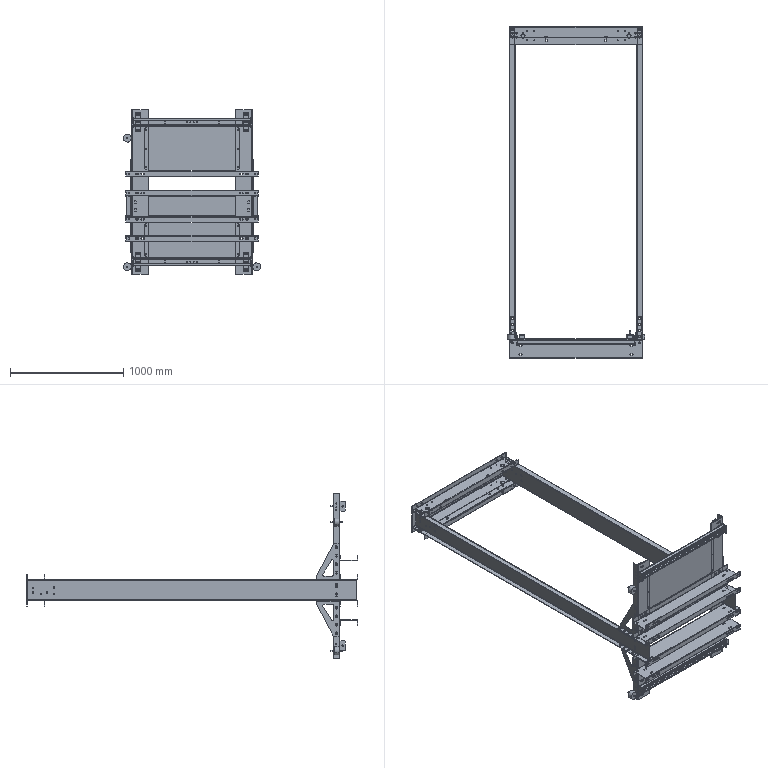Part | SolidWorks | 52 solids | 2434 faces | box 1212 x 2928 x 1450 mm | volume 26486943 mm3 | plane 1170 | cylinder 1144 | cone 120 | commonest cylinder face diameters 13 x308 14 x188 11 x76 12 x74 7 x52 6 x48